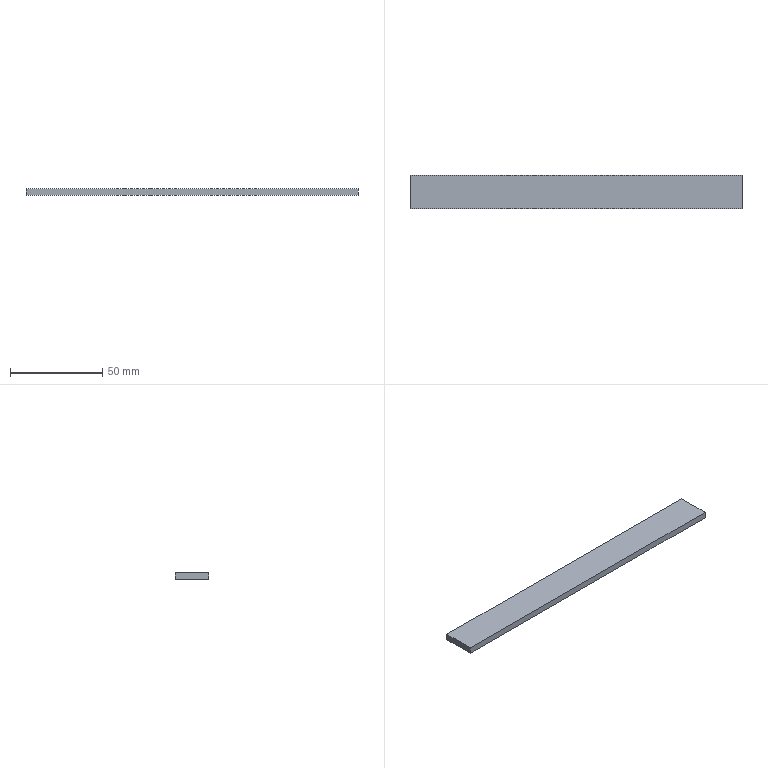Part | NX | 1 solid | 6 faces | box 180 x 18 x 3.6 mm | volume 11664 mm3 | plane 6
STEP:
#1=CARTESIAN_POINT('',(40.674,-586.499,2380.586));
#2=VERTEX_POINT('',#1);
#3=CARTESIAN_POINT('',(40.674,-604.499,2380.586));
#4=VERTEX_POINT('',#3);
#5=CARTESIAN_POINT('',(40.674,-604.499,2380.586));
#6=DIRECTION('',(0.,-1.,0.));
#7=VECTOR('',#6,1.);
#8=LINE('',#5,#7);
#9=EDGE_CURVE('',#2,#4,#8,.T.);
#10=ORIENTED_EDGE('',*,*,#9,.F.);
#11=CARTESIAN_POINT('',(40.674,-586.499,2376.986));
#12=VERTEX_POINT('',#11);
#13=CARTESIAN_POINT('',(40.674,-586.499,2380.586));
#14=DIRECTION('',(0.,0.,1.));
#15=VECTOR('',#14,1.);
#16=LINE('',#13,#15);
#17=EDGE_CURVE('',#12,#2,#16,.T.);
#18=ORIENTED_EDGE('',*,*,#17,.F.);
#19=CARTESIAN_POINT('',(40.674,-604.499,2376.986));
#20=VERTEX_POINT('',#19);
#21=CARTESIAN_POINT('',(40.674,-604.499,2376.986));
#22=DIRECTION('',(0.,1.,0.));
#23=VECTOR('',#22,1.);
#24=LINE('',#21,#23);
#25=EDGE_CURVE('',#20,#12,#24,.T.);
#26=ORIENTED_EDGE('',*,*,#25,.F.);
#27=CARTESIAN_POINT('',(40.674,-604.499,2380.586));
#28=DIRECTION('',(0.,0.,-1.));
#29=VECTOR('',#28,1.);
#30=LINE('',#27,#29);
#31=EDGE_CURVE('',#4,#20,#30,.T.);
#32=ORIENTED_EDGE('',*,*,#31,.F.);
#33=EDGE_LOOP('',(#10,#18,#26,#32));
#34=FACE_OUTER_BOUND('',#33,.T.);
#35=CARTESIAN_POINT('',(40.674,-586.499,2380.586));
#36=DIRECTION('',(-1.,0.,0.));
#37=DIRECTION('',(0.,0.,1.));
#38=AXIS2_PLACEMENT_3D('',#35,#36,#37);
#39=PLANE('',#38);
#40=ADVANCED_FACE('',(#34),#39,.T.);
#41=CARTESIAN_POINT('',(220.674,-586.499,2380.586));
#42=VERTEX_POINT('',#41);
#43=CARTESIAN_POINT('',(239.03,-586.499,2380.586));
#44=DIRECTION('',(-1.,0.,0.));
#45=VECTOR('',#44,1.);
#46=LINE('',#43,#45);
#47=EDGE_CURVE('',#42,#2,#46,.T.);
#48=ORIENTED_EDGE('',*,*,#47,.F.);
#49=CARTESIAN_POINT('',(220.674,-586.499,2376.986));
#50=VERTEX_POINT('',#49);
#51=CARTESIAN_POINT('',(220.674,-586.499,2380.586));
#52=DIRECTION('',(0.,0.,-1.));
#53=VECTOR('',#52,1.);
#54=LINE('',#51,#53);
#55=EDGE_CURVE('',#42,#50,#54,.T.);
#56=ORIENTED_EDGE('',*,*,#55,.T.);
#57=CARTESIAN_POINT('',(239.03,-586.499,2376.986));
#58=DIRECTION('',(-1.,0.,0.));
#59=VECTOR('',#58,1.);
#60=LINE('',#57,#59);
#61=EDGE_CURVE('',#50,#12,#60,.T.);
#62=ORIENTED_EDGE('',*,*,#61,.T.);
#63=ORIENTED_EDGE('',*,*,#17,.T.);
#64=EDGE_LOOP('',(#48,#56,#62,#63));
#65=FACE_OUTER_BOUND('',#64,.T.);
#66=CARTESIAN_POINT('',(239.03,-586.499,2380.586));
#67=DIRECTION('',(0.,-1.,0.));
#68=DIRECTION('',(0.,0.,-1.));
#69=AXIS2_PLACEMENT_3D('',#66,#67,#68);
#70=PLANE('',#69);
#71=ADVANCED_FACE('',(#65),#70,.F.);
#72=ORIENTED_EDGE('',*,*,#61,.F.);
#73=CARTESIAN_POINT('',(220.674,-604.499,2376.986));
#74=VERTEX_POINT('',#73);
#75=CARTESIAN_POINT('',(220.674,-604.499,2376.986));
#76=DIRECTION('',(0.,-1.,0.));
#77=VECTOR('',#76,1.);
#78=LINE('',#75,#77);
#79=EDGE_CURVE('',#50,#74,#78,.T.);
#80=ORIENTED_EDGE('',*,*,#79,.T.);
#81=CARTESIAN_POINT('',(239.03,-604.499,2376.986));
#82=DIRECTION('',(-1.,0.,0.));
#83=VECTOR('',#82,1.);
#84=LINE('',#81,#83);
#85=EDGE_CURVE('',#74,#20,#84,.T.);
#86=ORIENTED_EDGE('',*,*,#85,.T.);
#87=ORIENTED_EDGE('',*,*,#25,.T.);
#88=EDGE_LOOP('',(#72,#80,#86,#87));
#89=FACE_OUTER_BOUND('',#88,.T.);
#90=CARTESIAN_POINT('',(239.03,-604.499,2376.986));
#91=DIRECTION('',(0.,0.,1.));
#92=DIRECTION('',(1.,0.,0.));
#93=AXIS2_PLACEMENT_3D('',#90,#91,#92);
#94=PLANE('',#93);
#95=ADVANCED_FACE('',(#89),#94,.F.);
#96=ORIENTED_EDGE('',*,*,#85,.F.);
#97=CARTESIAN_POINT('',(220.674,-604.499,2380.586));
#98=VERTEX_POINT('',#97);
#99=CARTESIAN_POINT('',(220.674,-604.499,2380.586));
#100=DIRECTION('',(0.,0.,1.));
#101=VECTOR('',#100,1.);
#102=LINE('',#99,#101);
#103=EDGE_CURVE('',#74,#98,#102,.T.);
#104=ORIENTED_EDGE('',*,*,#103,.T.);
#105=CARTESIAN_POINT('',(239.03,-604.499,2380.586));
#106=DIRECTION('',(-1.,0.,0.));
#107=VECTOR('',#106,1.);
#108=LINE('',#105,#107);
#109=EDGE_CURVE('',#98,#4,#108,.T.);
#110=ORIENTED_EDGE('',*,*,#109,.T.);
#111=ORIENTED_EDGE('',*,*,#31,.T.);
#112=EDGE_LOOP('',(#96,#104,#110,#111));
#113=FACE_OUTER_BOUND('',#112,.T.);
#114=CARTESIAN_POINT('',(239.03,-604.499,2380.586));
#115=DIRECTION('',(0.,1.,0.));
#116=DIRECTION('',(0.,0.,1.));
#117=AXIS2_PLACEMENT_3D('',#114,#115,#116);
#118=PLANE('',#117);
#119=ADVANCED_FACE('',(#113),#118,.F.);
#120=ORIENTED_EDGE('',*,*,#109,.F.);
#121=CARTESIAN_POINT('',(220.674,-604.499,2380.586));
#122=DIRECTION('',(0.,1.,0.));
#123=VECTOR('',#122,1.);
#124=LINE('',#121,#123);
#125=EDGE_CURVE('',#98,#42,#124,.T.);
#126=ORIENTED_EDGE('',*,*,#125,.T.);
#127=ORIENTED_EDGE('',*,*,#47,.T.);
#128=ORIENTED_EDGE('',*,*,#9,.T.);
#129=EDGE_LOOP('',(#120,#126,#127,#128));
#130=FACE_OUTER_BOUND('',#129,.T.);
#131=CARTESIAN_POINT('',(239.03,-604.499,2380.586));
#132=DIRECTION('',(0.,0.,-1.));
#133=DIRECTION('',(-1.,0.,0.));
#134=AXIS2_PLACEMENT_3D('',#131,#132,#133);
#135=PLANE('',#134);
#136=ADVANCED_FACE('',(#130),#135,.F.);
#137=ORIENTED_EDGE('',*,*,#103,.F.);
#138=ORIENTED_EDGE('',*,*,#79,.F.);
#139=ORIENTED_EDGE('',*,*,#55,.F.);
#140=ORIENTED_EDGE('',*,*,#125,.F.);
#141=EDGE_LOOP('',(#137,#138,#139,#140));
#142=FACE_OUTER_BOUND('',#141,.T.);
#143=CARTESIAN_POINT('',(220.674,-484.499,2185.086));
#144=DIRECTION('',(-1.,0.,0.));
#145=DIRECTION('',(0.,0.,1.));
#146=AXIS2_PLACEMENT_3D('',#143,#144,#145);
#147=PLANE('',#146);
#148=ADVANCED_FACE('',(#142),#147,.F.);
#149=CLOSED_SHELL('',(#40,#71,#95,#119,#136,#148));
#150=MANIFOLD_SOLID_BREP('',#149);
#151=(LENGTH_UNIT()NAMED_UNIT(*)SI_UNIT(.MILLI.,.METRE.));
#152=UNCERTAINTY_MEASURE_WITH_UNIT(LENGTH_MEASURE(0.00002),#151,'','');
#153=(NAMED_UNIT(*)PLANE_ANGLE_UNIT()SI_UNIT($,.RADIAN.));
#154=PLANE_ANGLE_MEASURE_WITH_UNIT(PLANE_ANGLE_MEASURE(0.01745),#153);
#155=DIMENSIONAL_EXPONENTS(0.,0.,0.,0.,0.,0.,0.);
#156=(CONVERSION_BASED_UNIT('DEGREE',#154)NAMED_UNIT(#155)PLANE_ANGLE_UNIT());
#157=(NAMED_UNIT(*)SI_UNIT($,.STERADIAN.)SOLID_ANGLE_UNIT());
#158=(GEOMETRIC_REPRESENTATION_CONTEXT(3)GLOBAL_UNCERTAINTY_ASSIGNED_CONTEXT((#152))GLOBAL_UNIT_ASSIGNED_CONTEXT((#151,#156,#157))REPRESENTATION_CONTEXT('',''));
#159=ADVANCED_BREP_SHAPE_REPRESENTATION('',(#150),#158);